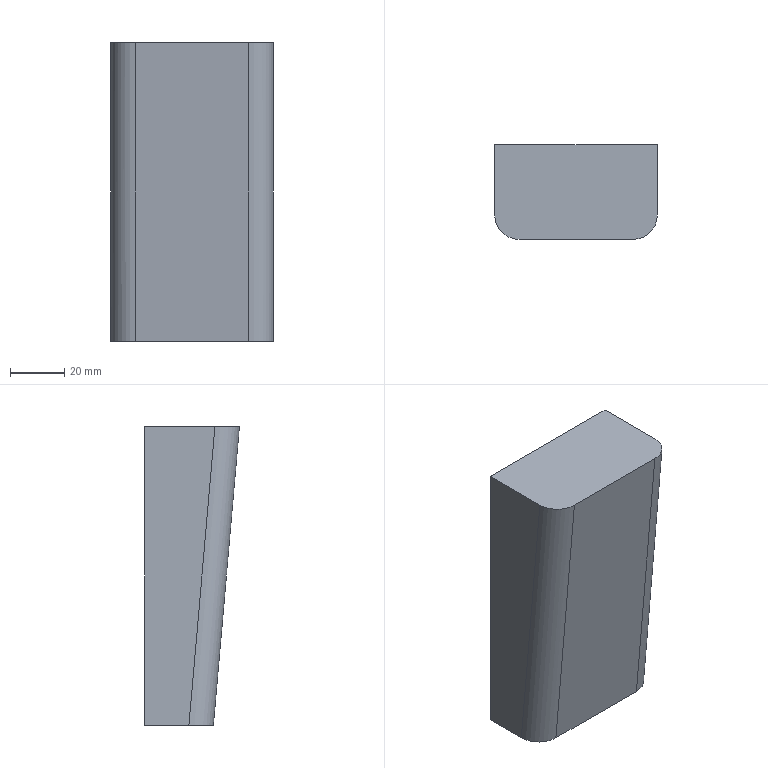Part | Creo | 1 solid | 8 faces | box 60 x 35 x 110 mm | volume 195403 mm3 | plane 6 | cylinder 2 | commonest cylinder face diameters 18 x2
STEP:
#1=CARTESIAN_POINT('',(0.,0.,0.));
#2=DIRECTION('',(0.,0.,1.));
#3=DIRECTION('',(1.,0.,0.));
#4=AXIS2_PLACEMENT_3D('',#1,#2,#3);
#5=CARTESIAN_POINT('',(-100.899,-334.593,-29.441));
#6=VERTEX_POINT('',#5);
#7=CARTESIAN_POINT('',(-100.899,-308.627,-29.441));
#8=VERTEX_POINT('',#7);
#9=CARTESIAN_POINT('',(-100.899,-334.593,-29.441));
#10=DIRECTION('',(0.,1.,0.));
#11=VECTOR('',#10,25.966);
#12=LINE('',#9,#11);
#13=EDGE_CURVE('',#6,#8,#12,.T.);
#14=ORIENTED_EDGE('',*,*,#13,.T.);
#15=CARTESIAN_POINT('',(-100.899,-308.627,-139.441));
#16=VERTEX_POINT('',#15);
#17=CARTESIAN_POINT('',(-100.899,-308.627,-29.441));
#18=DIRECTION('',(0.,0.,-1.));
#19=VECTOR('',#18,110.);
#20=LINE('',#17,#19);
#21=EDGE_CURVE('',#8,#16,#20,.T.);
#22=ORIENTED_EDGE('',*,*,#21,.T.);
#23=CARTESIAN_POINT('',(-100.899,-324.969,-139.441));
#24=VERTEX_POINT('',#23);
#25=CARTESIAN_POINT('',(-100.899,-324.969,-139.441));
#26=DIRECTION('',(0.,1.,0.));
#27=VECTOR('',#26,16.342);
#28=LINE('',#25,#27);
#29=EDGE_CURVE('',#24,#16,#28,.T.);
#30=ORIENTED_EDGE('',*,*,#29,.F.);
#31=CARTESIAN_POINT('',(-100.899,-334.593,-29.441));
#32=DIRECTION('',(0.,0.08716,-0.9962));
#33=VECTOR('',#32,110.42);
#34=LINE('',#31,#33);
#35=EDGE_CURVE('',#6,#24,#34,.T.);
#36=ORIENTED_EDGE('',*,*,#35,.F.);
#37=EDGE_LOOP('',(#14,#22,#30,#36));
#38=FACE_OUTER_BOUND('',#37,.F.);
#39=CARTESIAN_POINT('',(-100.899,-308.627,-109.441));
#40=DIRECTION('',(1.,0.,0.));
#41=DIRECTION('',(0.,0.,-1.));
#42=AXIS2_PLACEMENT_3D('',#39,#40,#41);
#43=PLANE('',#42);
#44=ADVANCED_FACE('',(#38),#43,.T.);
#45=CARTESIAN_POINT('',(-151.899,-343.627,-29.441));
#46=VERTEX_POINT('',#45);
#47=CARTESIAN_POINT('',(-109.899,-343.627,-29.441));
#48=VERTEX_POINT('',#47);
#49=CARTESIAN_POINT('',(-151.899,-343.627,-29.441));
#50=DIRECTION('',(1.,0.,0.));
#51=VECTOR('',#50,42.);
#52=LINE('',#49,#51);
#53=EDGE_CURVE('',#46,#48,#52,.T.);
#54=ORIENTED_EDGE('',*,*,#53,.F.);
#55=CARTESIAN_POINT('',(-160.899,-334.593,-29.441));
#56=VERTEX_POINT('',#55);
#57=CARTESIAN_POINT('',(-151.899,-343.627,-29.441));
#58=CARTESIAN_POINT('',(-152.651,-343.627,-29.441));
#59=CARTESIAN_POINT('',(-153.975,-343.449,-29.441));
#60=CARTESIAN_POINT('',(-156.202,-342.671,-29.441));
#61=CARTESIAN_POINT('',(-158.394,-341.105,-29.441));
#62=CARTESIAN_POINT('',(-159.95,-338.904,-29.441));
#63=CARTESIAN_POINT('',(-160.722,-336.671,-29.441));
#64=CARTESIAN_POINT('',(-160.899,-335.345,-29.441));
#65=CARTESIAN_POINT('',(-160.899,-334.593,-29.441));
#66=B_SPLINE_CURVE_WITH_KNOTS('',3,(#57,#58,#59,#60,#61,#62,#63,#64,#65),.UNSPECIFIED.,.F.,.F.,(4,1,1,1,1,1,4),(0.,0.125,0.25,0.5,0.75,0.875,1.),.UNSPECIFIED.);
#67=EDGE_CURVE('',#46,#56,#66,.T.);
#68=ORIENTED_EDGE('',*,*,#67,.T.);
#69=CARTESIAN_POINT('',(-160.899,-308.627,-29.441));
#70=VERTEX_POINT('',#69);
#71=CARTESIAN_POINT('',(-160.899,-308.627,-29.441));
#72=DIRECTION('',(0.,-1.,0.));
#73=VECTOR('',#72,25.966);
#74=LINE('',#71,#73);
#75=EDGE_CURVE('',#70,#56,#74,.T.);
#76=ORIENTED_EDGE('',*,*,#75,.F.);
#77=CARTESIAN_POINT('',(-100.899,-308.627,-29.441));
#78=DIRECTION('',(-1.,0.,0.));
#79=VECTOR('',#78,60.);
#80=LINE('',#77,#79);
#81=EDGE_CURVE('',#8,#70,#80,.T.);
#82=ORIENTED_EDGE('',*,*,#81,.F.);
#83=ORIENTED_EDGE('',*,*,#13,.F.);
#84=CARTESIAN_POINT('',(-100.899,-334.593,-29.441));
#85=CARTESIAN_POINT('',(-100.899,-335.345,-29.441));
#86=CARTESIAN_POINT('',(-101.076,-336.671,-29.441));
#87=CARTESIAN_POINT('',(-101.848,-338.904,-29.441));
#88=CARTESIAN_POINT('',(-103.405,-341.105,-29.441));
#89=CARTESIAN_POINT('',(-105.596,-342.671,-29.441));
#90=CARTESIAN_POINT('',(-107.823,-343.449,-29.441));
#91=CARTESIAN_POINT('',(-109.148,-343.627,-29.441));
#92=CARTESIAN_POINT('',(-109.899,-343.627,-29.441));
#93=B_SPLINE_CURVE_WITH_KNOTS('',3,(#84,#85,#86,#87,#88,#89,#90,#91,#92),.UNSPECIFIED.,.F.,.F.,(4,1,1,1,1,1,4),(0.,0.125,0.25,0.5,0.75,0.875,1.),.UNSPECIFIED.);
#94=EDGE_CURVE('',#6,#48,#93,.T.);
#95=ORIENTED_EDGE('',*,*,#94,.T.);
#96=EDGE_LOOP('',(#54,#68,#76,#82,#83,#95));
#97=FACE_OUTER_BOUND('',#96,.F.);
#98=CARTESIAN_POINT('',(-53.899,-338.627,-29.441));
#99=DIRECTION('',(0.,0.,1.));
#100=DIRECTION('',(1.,0.,0.));
#101=AXIS2_PLACEMENT_3D('',#98,#99,#100);
#102=PLANE('',#101);
#103=ADVANCED_FACE('',(#97),#102,.T.);
#104=CARTESIAN_POINT('',(-151.899,-334.004,-139.441));
#105=VERTEX_POINT('',#104);
#106=CARTESIAN_POINT('',(-109.899,-334.004,-139.441));
#107=VERTEX_POINT('',#106);
#108=CARTESIAN_POINT('',(-151.899,-334.004,-139.441));
#109=DIRECTION('',(1.,0.,0.));
#110=VECTOR('',#109,42.);
#111=LINE('',#108,#110);
#112=EDGE_CURVE('',#105,#107,#111,.T.);
#113=ORIENTED_EDGE('',*,*,#112,.F.);
#114=CARTESIAN_POINT('',(-151.899,-334.004,-139.441));
#115=DIRECTION('',(0.,-0.08716,0.9962));
#116=VECTOR('',#115,110.42);
#117=LINE('',#114,#116);
#118=EDGE_CURVE('',#105,#46,#117,.T.);
#119=ORIENTED_EDGE('',*,*,#118,.T.);
#120=ORIENTED_EDGE('',*,*,#53,.T.);
#121=CARTESIAN_POINT('',(-109.899,-343.627,-29.441));
#122=DIRECTION('',(0.,0.08716,-0.9962));
#123=VECTOR('',#122,110.42);
#124=LINE('',#121,#123);
#125=EDGE_CURVE('',#48,#107,#124,.T.);
#126=ORIENTED_EDGE('',*,*,#125,.T.);
#127=EDGE_LOOP('',(#113,#119,#120,#126));
#128=FACE_OUTER_BOUND('',#127,.F.);
#129=CARTESIAN_POINT('',(-53.899,-343.627,-29.441));
#130=DIRECTION('',(0.,0.9962,0.08716));
#131=DIRECTION('',(0.,-0.08716,0.9962));
#132=AXIS2_PLACEMENT_3D('',#129,#130,#131);
#133=PLANE('',#132);
#134=ADVANCED_FACE('',(#128),#133,.F.);
#135=ORIENTED_EDGE('',*,*,#29,.T.);
#136=CARTESIAN_POINT('',(-160.899,-308.627,-139.441));
#137=VERTEX_POINT('',#136);
#138=CARTESIAN_POINT('',(-100.899,-308.627,-139.441));
#139=DIRECTION('',(-1.,0.,0.));
#140=VECTOR('',#139,60.);
#141=LINE('',#138,#140);
#142=EDGE_CURVE('',#16,#137,#141,.T.);
#143=ORIENTED_EDGE('',*,*,#142,.T.);
#144=CARTESIAN_POINT('',(-160.899,-324.969,-139.441));
#145=VERTEX_POINT('',#144);
#146=CARTESIAN_POINT('',(-160.899,-308.627,-139.441));
#147=DIRECTION('',(0.,-1.,0.));
#148=VECTOR('',#147,16.342);
#149=LINE('',#146,#148);
#150=EDGE_CURVE('',#137,#145,#149,.T.);
#151=ORIENTED_EDGE('',*,*,#150,.T.);
#152=CARTESIAN_POINT('',(-160.899,-324.969,-139.441));
#153=CARTESIAN_POINT('',(-160.899,-325.721,-139.441));
#154=CARTESIAN_POINT('',(-160.722,-327.047,-139.441));
#155=CARTESIAN_POINT('',(-159.95,-329.28,-139.441));
#156=CARTESIAN_POINT('',(-158.394,-331.481,-139.441));
#157=CARTESIAN_POINT('',(-156.202,-333.047,-139.441));
#158=CARTESIAN_POINT('',(-153.975,-333.825,-139.441));
#159=CARTESIAN_POINT('',(-152.651,-334.004,-139.441));
#160=CARTESIAN_POINT('',(-151.899,-334.004,-139.441));
#161=B_SPLINE_CURVE_WITH_KNOTS('',3,(#152,#153,#154,#155,#156,#157,#158,#159,#160),.UNSPECIFIED.,.F.,.F.,(4,1,1,1,1,1,4),(0.,0.125,0.25,0.5,0.75,0.875,1.),.UNSPECIFIED.);
#162=EDGE_CURVE('',#145,#105,#161,.T.);
#163=ORIENTED_EDGE('',*,*,#162,.T.);
#164=ORIENTED_EDGE('',*,*,#112,.T.);
#165=CARTESIAN_POINT('',(-109.899,-334.004,-139.441));
#166=CARTESIAN_POINT('',(-109.148,-334.004,-139.441));
#167=CARTESIAN_POINT('',(-107.823,-333.825,-139.441));
#168=CARTESIAN_POINT('',(-105.596,-333.047,-139.441));
#169=CARTESIAN_POINT('',(-103.405,-331.481,-139.441));
#170=CARTESIAN_POINT('',(-101.848,-329.28,-139.441));
#171=CARTESIAN_POINT('',(-101.076,-327.047,-139.441));
#172=CARTESIAN_POINT('',(-100.899,-325.721,-139.441));
#173=CARTESIAN_POINT('',(-100.899,-324.969,-139.441));
#174=B_SPLINE_CURVE_WITH_KNOTS('',3,(#165,#166,#167,#168,#169,#170,#171,#172,#173),.UNSPECIFIED.,.F.,.F.,(4,1,1,1,1,1,4),(0.,0.125,0.25,0.5,0.75,0.875,1.),.UNSPECIFIED.);
#175=EDGE_CURVE('',#107,#24,#174,.T.);
#176=ORIENTED_EDGE('',*,*,#175,.T.);
#177=EDGE_LOOP('',(#135,#143,#151,#163,#164,#176));
#178=FACE_OUTER_BOUND('',#177,.F.);
#179=CARTESIAN_POINT('',(-53.899,-338.627,-139.441));
#180=DIRECTION('',(0.,0.,1.));
#181=DIRECTION('',(1.,0.,0.));
#182=AXIS2_PLACEMENT_3D('',#179,#180,#181);
#183=PLANE('',#182);
#184=ADVANCED_FACE('',(#178),#183,.F.);
#185=ORIENTED_EDGE('',*,*,#81,.T.);
#186=CARTESIAN_POINT('',(-160.899,-308.627,-29.441));
#187=DIRECTION('',(0.,0.,-1.));
#188=VECTOR('',#187,110.);
#189=LINE('',#186,#188);
#190=EDGE_CURVE('',#70,#137,#189,.T.);
#191=ORIENTED_EDGE('',*,*,#190,.T.);
#192=ORIENTED_EDGE('',*,*,#142,.F.);
#193=ORIENTED_EDGE('',*,*,#21,.F.);
#194=EDGE_LOOP('',(#185,#191,#192,#193));
#195=FACE_OUTER_BOUND('',#194,.F.);
#196=CARTESIAN_POINT('',(-160.899,-308.627,-109.441));
#197=DIRECTION('',(0.,1.,0.));
#198=DIRECTION('',(0.,0.,1.));
#199=AXIS2_PLACEMENT_3D('',#196,#197,#198);
#200=PLANE('',#199);
#201=ADVANCED_FACE('',(#195),#200,.T.);
#202=ORIENTED_EDGE('',*,*,#150,.F.);
#203=ORIENTED_EDGE('',*,*,#190,.F.);
#204=ORIENTED_EDGE('',*,*,#75,.T.);
#205=CARTESIAN_POINT('',(-160.899,-324.969,-139.441));
#206=DIRECTION('',(0.,-0.08716,0.9962));
#207=VECTOR('',#206,110.42);
#208=LINE('',#205,#207);
#209=EDGE_CURVE('',#145,#56,#208,.T.);
#210=ORIENTED_EDGE('',*,*,#209,.F.);
#211=EDGE_LOOP('',(#202,#203,#204,#210));
#212=FACE_OUTER_BOUND('',#211,.F.);
#213=CARTESIAN_POINT('',(-160.899,-338.627,-109.441));
#214=DIRECTION('',(-1.,0.,0.));
#215=DIRECTION('',(0.,0.,1.));
#216=AXIS2_PLACEMENT_3D('',#213,#214,#215);
#217=PLANE('',#216);
#218=ADVANCED_FACE('',(#212),#217,.T.);
#219=ORIENTED_EDGE('',*,*,#162,.F.);
#220=ORIENTED_EDGE('',*,*,#209,.T.);
#221=ORIENTED_EDGE('',*,*,#67,.F.);
#222=ORIENTED_EDGE('',*,*,#118,.F.);
#223=EDGE_LOOP('',(#219,#220,#221,#222));
#224=FACE_OUTER_BOUND('',#223,.F.);
#225=CARTESIAN_POINT('',(-151.899,-327.678,-108.483));
#226=DIRECTION('',(0.,0.08716,-0.9962));
#227=DIRECTION('',(0.,0.9962,0.08716));
#228=AXIS2_PLACEMENT_3D('',#225,#226,#227);
#229=CYLINDRICAL_SURFACE('',#228,9.);
#230=ADVANCED_FACE('',(#224),#229,.T.);
#231=ORIENTED_EDGE('',*,*,#175,.F.);
#232=ORIENTED_EDGE('',*,*,#125,.F.);
#233=ORIENTED_EDGE('',*,*,#94,.F.);
#234=ORIENTED_EDGE('',*,*,#35,.T.);
#235=EDGE_LOOP('',(#231,#232,#233,#234));
#236=FACE_OUTER_BOUND('',#235,.F.);
#237=CARTESIAN_POINT('',(-109.899,-334.662,-28.657));
#238=DIRECTION('',(0.,0.08716,-0.9962));
#239=DIRECTION('',(0.,0.9962,0.08716));
#240=AXIS2_PLACEMENT_3D('',#237,#238,#239);
#241=CYLINDRICAL_SURFACE('',#240,9.);
#242=ADVANCED_FACE('',(#236),#241,.T.);
#243=CLOSED_SHELL('',(#44,#103,#134,#184,#201,#218,#230,#242));
#244=MANIFOLD_SOLID_BREP('',#243);
#245=(LENGTH_UNIT()NAMED_UNIT(*)SI_UNIT(.MILLI.,.METRE.));
#246=UNCERTAINTY_MEASURE_WITH_UNIT(LENGTH_MEASURE(0.01314),#245,'','');
#247=(NAMED_UNIT(*)PLANE_ANGLE_UNIT()SI_UNIT($,.RADIAN.));
#248=PLANE_ANGLE_MEASURE_WITH_UNIT(PLANE_ANGLE_MEASURE(0.01745),#247);
#249=(CONVERSION_BASED_UNIT('DEGREE',#248)NAMED_UNIT(*)PLANE_ANGLE_UNIT());
#250=(NAMED_UNIT(*)SI_UNIT($,.STERADIAN.)SOLID_ANGLE_UNIT());
#251=(GEOMETRIC_REPRESENTATION_CONTEXT(3)GLOBAL_UNCERTAINTY_ASSIGNED_CONTEXT((#246))GLOBAL_UNIT_ASSIGNED_CONTEXT((#245,#249,#250))REPRESENTATION_CONTEXT('',''));
#252=ADVANCED_BREP_SHAPE_REPRESENTATION('',(#4,#244),#251);